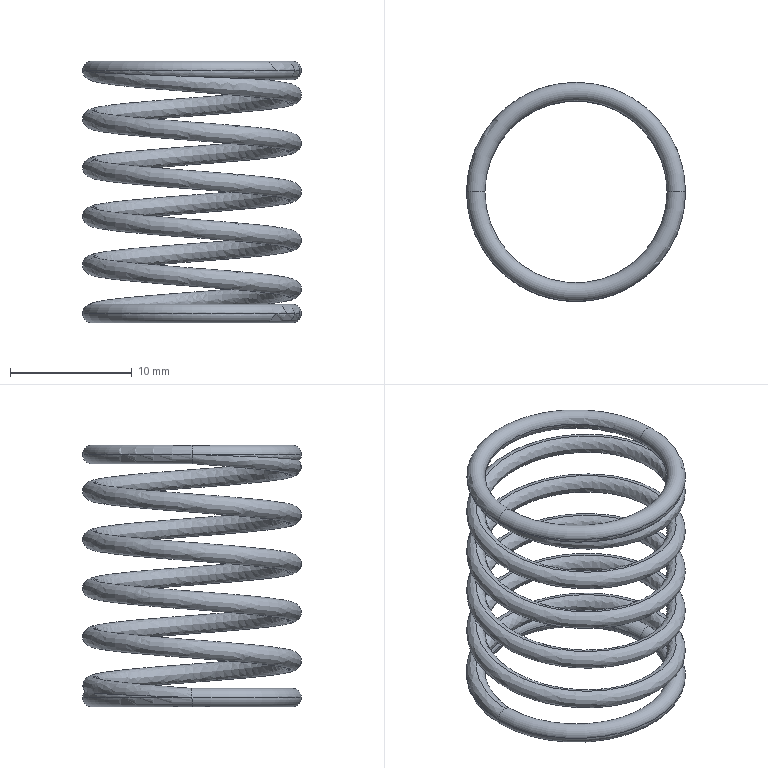Part | SolidWorks | features BaseBody 1 | 1 solid | 10 faces | box 18.005 x 18.005 x 21.505 mm | volume 615.294 mm3 | torus 8 | spline 2